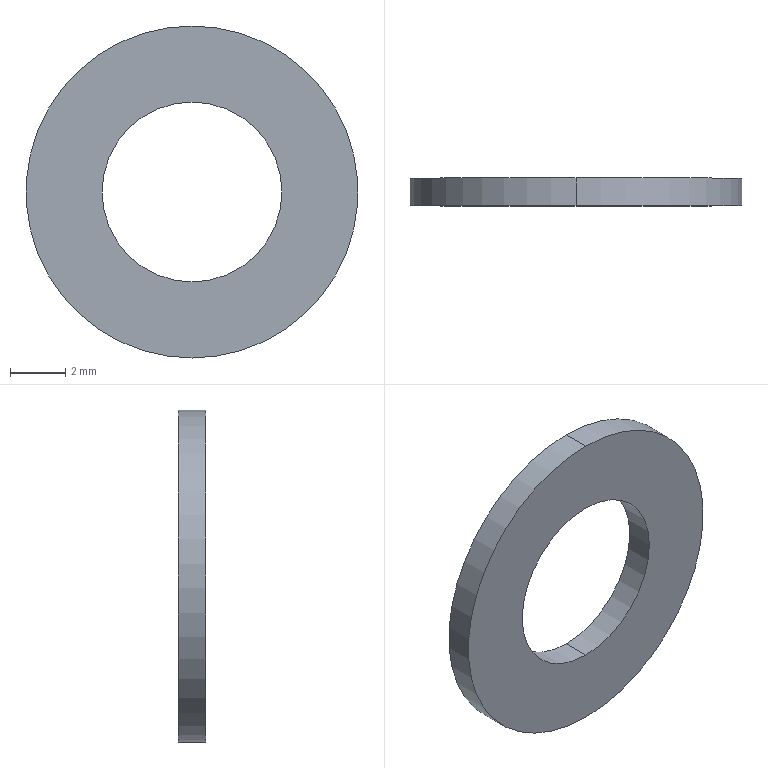Part | STEP file | Washer A | 1 solid | 6 faces | box 12 x 1 x 12 mm | volume 79.914 mm3 | cylinder 4 | plane 2 | commonest cylinder face diameters 6.5 x2 12 x2
STEP:
#1=CARTESIAN_POINT('',(0.,0.,0.));
#2=DIRECTION('',(0.,0.,1.));
#3=DIRECTION('',(1.,0.,0.));
#4=AXIS2_PLACEMENT_3D('',#1,#2,#3);
#5=CARTESIAN_POINT('',(0.,-1.,3.25));
#6=VERTEX_POINT('',#5);
#7=CARTESIAN_POINT('',(0.,0.,3.25));
#8=VERTEX_POINT('',#7);
#9=CARTESIAN_POINT('',(0.,-1.,3.25));
#10=DIRECTION('',(0.,1.,0.));
#11=VECTOR('',#10,1.);
#12=LINE('',#9,#11);
#13=CARTESIAN_POINT('',(0.,-1.,0.));
#14=DIRECTION('',(0.,1.,0.));
#15=DIRECTION('',(0.,0.,1.));
#16=AXIS2_PLACEMENT_3D('',#13,#14,#15);
#17=CYLINDRICAL_SURFACE('',#16,3.25);
#18=CARTESIAN_POINT('',(6.283,0.));
#19=DIRECTION('',(0.,1.));
#20=VECTOR('',#19,1.);
#21=LINE('',#18,#20);
#22=(GEOMETRIC_REPRESENTATION_CONTEXT(2)PARAMETRIC_REPRESENTATION_CONTEXT()REPRESENTATION_CONTEXT('',''));
#23=DEFINITIONAL_REPRESENTATION('',(#21),#22);
#24=PCURVE('',#17,#23);
#25=CARTESIAN_POINT('',(0.,-1.,0.));
#26=DIRECTION('',(0.,1.,0.));
#27=DIRECTION('',(0.,0.,1.));
#28=AXIS2_PLACEMENT_3D('',#25,#26,#27);
#29=CYLINDRICAL_SURFACE('',#28,3.25);
#30=CARTESIAN_POINT('',(0.,0.));
#31=DIRECTION('',(0.,1.));
#32=VECTOR('',#31,1.);
#33=LINE('',#30,#32);
#34=(GEOMETRIC_REPRESENTATION_CONTEXT(2)PARAMETRIC_REPRESENTATION_CONTEXT()REPRESENTATION_CONTEXT('',''));
#35=DEFINITIONAL_REPRESENTATION('',(#33),#34);
#36=PCURVE('',#29,#35);
#37=SURFACE_CURVE('',#12,(#24,#36),.PCURVE_S1.);
#38=EDGE_CURVE('',#6,#8,#37,.T.);
#39=ORIENTED_EDGE('',*,*,#38,.T.);
#40=CARTESIAN_POINT('',(0.,0.,-3.25));
#41=VERTEX_POINT('',#40);
#42=CARTESIAN_POINT('',(0.,0.,0.));
#43=DIRECTION('',(0.,1.,0.));
#44=DIRECTION('',(0.,0.,1.));
#45=AXIS2_PLACEMENT_3D('',#42,#43,#44);
#46=CIRCLE('',#45,3.25);
#47=CARTESIAN_POINT('',(0.,1.));
#48=DIRECTION('',(1.,0.));
#49=VECTOR('',#48,1.);
#50=LINE('',#47,#49);
#51=(GEOMETRIC_REPRESENTATION_CONTEXT(2)PARAMETRIC_REPRESENTATION_CONTEXT()REPRESENTATION_CONTEXT('',''));
#52=DEFINITIONAL_REPRESENTATION('',(#50),#51);
#53=PCURVE('',#17,#52);
#54=CARTESIAN_POINT('',(0.,0.,0.));
#55=DIRECTION('',(0.,1.,0.));
#56=DIRECTION('',(0.,0.,1.));
#57=AXIS2_PLACEMENT_3D('',#54,#55,#56);
#58=PLANE('',#57);
#59=CARTESIAN_POINT('',(0.,0.));
#60=DIRECTION('',(1.,0.));
#61=AXIS2_PLACEMENT_2D('',#59,#60);
#62=CIRCLE('',#61,3.25);
#63=(GEOMETRIC_REPRESENTATION_CONTEXT(2)PARAMETRIC_REPRESENTATION_CONTEXT()REPRESENTATION_CONTEXT('',''));
#64=DEFINITIONAL_REPRESENTATION('',(#62),#63);
#65=PCURVE('',#58,#64);
#66=SURFACE_CURVE('',#46,(#53,#65),.PCURVE_S1.);
#67=EDGE_CURVE('',#41,#8,#66,.T.);
#68=ORIENTED_EDGE('',*,*,#67,.F.);
#69=CARTESIAN_POINT('',(0.,-1.,-3.25));
#70=VERTEX_POINT('',#69);
#71=CARTESIAN_POINT('',(0.,-1.,-3.25));
#72=DIRECTION('',(0.,1.,0.));
#73=VECTOR('',#72,1.);
#74=LINE('',#71,#73);
#75=CARTESIAN_POINT('',(3.142,0.));
#76=DIRECTION('',(0.,1.));
#77=VECTOR('',#76,1.);
#78=LINE('',#75,#77);
#79=(GEOMETRIC_REPRESENTATION_CONTEXT(2)PARAMETRIC_REPRESENTATION_CONTEXT()REPRESENTATION_CONTEXT('',''));
#80=DEFINITIONAL_REPRESENTATION('',(#78),#79);
#81=PCURVE('',#17,#80);
#82=CARTESIAN_POINT('',(3.142,0.));
#83=DIRECTION('',(0.,1.));
#84=VECTOR('',#83,1.);
#85=LINE('',#82,#84);
#86=(GEOMETRIC_REPRESENTATION_CONTEXT(2)PARAMETRIC_REPRESENTATION_CONTEXT()REPRESENTATION_CONTEXT('',''));
#87=DEFINITIONAL_REPRESENTATION('',(#85),#86);
#88=PCURVE('',#29,#87);
#89=SURFACE_CURVE('',#74,(#81,#88),.PCURVE_S1.);
#90=EDGE_CURVE('',#70,#41,#89,.T.);
#91=ORIENTED_EDGE('',*,*,#90,.F.);
#92=CARTESIAN_POINT('',(0.,-1.,0.));
#93=DIRECTION('',(0.,1.,0.));
#94=DIRECTION('',(0.,0.,1.));
#95=AXIS2_PLACEMENT_3D('',#92,#93,#94);
#96=CIRCLE('',#95,3.25);
#97=CARTESIAN_POINT('',(0.,0.));
#98=DIRECTION('',(1.,0.));
#99=VECTOR('',#98,1.);
#100=LINE('',#97,#99);
#101=(GEOMETRIC_REPRESENTATION_CONTEXT(2)PARAMETRIC_REPRESENTATION_CONTEXT()REPRESENTATION_CONTEXT('',''));
#102=DEFINITIONAL_REPRESENTATION('',(#100),#101);
#103=PCURVE('',#17,#102);
#104=CARTESIAN_POINT('',(0.,-1.,0.));
#105=DIRECTION('',(0.,1.,0.));
#106=DIRECTION('',(0.,0.,1.));
#107=AXIS2_PLACEMENT_3D('',#104,#105,#106);
#108=PLANE('',#107);
#109=CARTESIAN_POINT('',(0.,0.));
#110=DIRECTION('',(1.,0.));
#111=AXIS2_PLACEMENT_2D('',#109,#110);
#112=CIRCLE('',#111,3.25);
#113=(GEOMETRIC_REPRESENTATION_CONTEXT(2)PARAMETRIC_REPRESENTATION_CONTEXT()REPRESENTATION_CONTEXT('',''));
#114=DEFINITIONAL_REPRESENTATION('',(#112),#113);
#115=PCURVE('',#108,#114);
#116=SURFACE_CURVE('',#96,(#103,#115),.PCURVE_S1.);
#117=EDGE_CURVE('',#70,#6,#116,.T.);
#118=ORIENTED_EDGE('',*,*,#117,.T.);
#119=EDGE_LOOP('',(#39,#68,#91,#118));
#120=FACE_BOUND('',#119,.F.);
#121=ADVANCED_FACE('',(#120),#17,.F.);
#122=CARTESIAN_POINT('',(0.,-1.,6.));
#123=VERTEX_POINT('',#122);
#124=CARTESIAN_POINT('',(0.,-1.,-6.));
#125=VERTEX_POINT('',#124);
#126=CARTESIAN_POINT('',(0.,-1.,0.));
#127=DIRECTION('',(0.,1.,0.));
#128=DIRECTION('',(0.,0.,1.));
#129=AXIS2_PLACEMENT_3D('',#126,#127,#128);
#130=CIRCLE('',#129,6.);
#131=CARTESIAN_POINT('',(0.,-1.,0.));
#132=DIRECTION('',(0.,1.,0.));
#133=DIRECTION('',(0.,0.,1.));
#134=AXIS2_PLACEMENT_3D('',#131,#132,#133);
#135=CYLINDRICAL_SURFACE('',#134,6.);
#136=CARTESIAN_POINT('',(0.,0.));
#137=DIRECTION('',(1.,0.));
#138=VECTOR('',#137,1.);
#139=LINE('',#136,#138);
#140=(GEOMETRIC_REPRESENTATION_CONTEXT(2)PARAMETRIC_REPRESENTATION_CONTEXT()REPRESENTATION_CONTEXT('',''));
#141=DEFINITIONAL_REPRESENTATION('',(#139),#140);
#142=PCURVE('',#135,#141);
#143=CARTESIAN_POINT('',(0.,0.));
#144=DIRECTION('',(1.,0.));
#145=AXIS2_PLACEMENT_2D('',#143,#144);
#146=CIRCLE('',#145,6.);
#147=(GEOMETRIC_REPRESENTATION_CONTEXT(2)PARAMETRIC_REPRESENTATION_CONTEXT()REPRESENTATION_CONTEXT('',''));
#148=DEFINITIONAL_REPRESENTATION('',(#146),#147);
#149=PCURVE('',#108,#148);
#150=SURFACE_CURVE('',#130,(#142,#149),.PCURVE_S1.);
#151=EDGE_CURVE('',#123,#125,#150,.T.);
#152=ORIENTED_EDGE('',*,*,#151,.T.);
#153=CARTESIAN_POINT('',(0.,0.,-6.));
#154=VERTEX_POINT('',#153);
#155=CARTESIAN_POINT('',(0.,-1.,-6.));
#156=DIRECTION('',(0.,1.,0.));
#157=VECTOR('',#156,1.);
#158=LINE('',#155,#157);
#159=CARTESIAN_POINT('',(3.142,0.));
#160=DIRECTION('',(0.,1.));
#161=VECTOR('',#160,1.);
#162=LINE('',#159,#161);
#163=(GEOMETRIC_REPRESENTATION_CONTEXT(2)PARAMETRIC_REPRESENTATION_CONTEXT()REPRESENTATION_CONTEXT('',''));
#164=DEFINITIONAL_REPRESENTATION('',(#162),#163);
#165=PCURVE('',#135,#164);
#166=CARTESIAN_POINT('',(0.,-1.,0.));
#167=DIRECTION('',(0.,1.,0.));
#168=DIRECTION('',(0.,0.,1.));
#169=AXIS2_PLACEMENT_3D('',#166,#167,#168);
#170=CYLINDRICAL_SURFACE('',#169,6.);
#171=CARTESIAN_POINT('',(3.142,0.));
#172=DIRECTION('',(0.,1.));
#173=VECTOR('',#172,1.);
#174=LINE('',#171,#173);
#175=(GEOMETRIC_REPRESENTATION_CONTEXT(2)PARAMETRIC_REPRESENTATION_CONTEXT()REPRESENTATION_CONTEXT('',''));
#176=DEFINITIONAL_REPRESENTATION('',(#174),#175);
#177=PCURVE('',#170,#176);
#178=SURFACE_CURVE('',#158,(#165,#177),.PCURVE_S1.);
#179=EDGE_CURVE('',#125,#154,#178,.T.);
#180=ORIENTED_EDGE('',*,*,#179,.T.);
#181=CARTESIAN_POINT('',(0.,0.,6.));
#182=VERTEX_POINT('',#181);
#183=CARTESIAN_POINT('',(0.,0.,0.));
#184=DIRECTION('',(0.,1.,0.));
#185=DIRECTION('',(0.,0.,1.));
#186=AXIS2_PLACEMENT_3D('',#183,#184,#185);
#187=CIRCLE('',#186,6.);
#188=CARTESIAN_POINT('',(0.,1.));
#189=DIRECTION('',(1.,0.));
#190=VECTOR('',#189,1.);
#191=LINE('',#188,#190);
#192=(GEOMETRIC_REPRESENTATION_CONTEXT(2)PARAMETRIC_REPRESENTATION_CONTEXT()REPRESENTATION_CONTEXT('',''));
#193=DEFINITIONAL_REPRESENTATION('',(#191),#192);
#194=PCURVE('',#135,#193);
#195=CARTESIAN_POINT('',(0.,0.));
#196=DIRECTION('',(1.,0.));
#197=AXIS2_PLACEMENT_2D('',#195,#196);
#198=CIRCLE('',#197,6.);
#199=(GEOMETRIC_REPRESENTATION_CONTEXT(2)PARAMETRIC_REPRESENTATION_CONTEXT()REPRESENTATION_CONTEXT('',''));
#200=DEFINITIONAL_REPRESENTATION('',(#198),#199);
#201=PCURVE('',#58,#200);
#202=SURFACE_CURVE('',#187,(#194,#201),.PCURVE_S1.);
#203=EDGE_CURVE('',#182,#154,#202,.T.);
#204=ORIENTED_EDGE('',*,*,#203,.F.);
#205=CARTESIAN_POINT('',(0.,-1.,6.));
#206=DIRECTION('',(0.,1.,0.));
#207=VECTOR('',#206,1.);
#208=LINE('',#205,#207);
#209=CARTESIAN_POINT('',(0.,0.));
#210=DIRECTION('',(0.,1.));
#211=VECTOR('',#210,1.);
#212=LINE('',#209,#211);
#213=(GEOMETRIC_REPRESENTATION_CONTEXT(2)PARAMETRIC_REPRESENTATION_CONTEXT()REPRESENTATION_CONTEXT('',''));
#214=DEFINITIONAL_REPRESENTATION('',(#212),#213);
#215=PCURVE('',#135,#214);
#216=CARTESIAN_POINT('',(6.283,0.));
#217=DIRECTION('',(0.,1.));
#218=VECTOR('',#217,1.);
#219=LINE('',#216,#218);
#220=(GEOMETRIC_REPRESENTATION_CONTEXT(2)PARAMETRIC_REPRESENTATION_CONTEXT()REPRESENTATION_CONTEXT('',''));
#221=DEFINITIONAL_REPRESENTATION('',(#219),#220);
#222=PCURVE('',#170,#221);
#223=SURFACE_CURVE('',#208,(#215,#222),.PCURVE_S1.);
#224=EDGE_CURVE('',#123,#182,#223,.T.);
#225=ORIENTED_EDGE('',*,*,#224,.F.);
#226=EDGE_LOOP('',(#152,#180,#204,#225));
#227=FACE_BOUND('',#226,.T.);
#228=ADVANCED_FACE('',(#227),#135,.T.);
#229=ORIENTED_EDGE('',*,*,#179,.F.);
#230=CARTESIAN_POINT('',(0.,-1.,0.));
#231=DIRECTION('',(0.,1.,0.));
#232=DIRECTION('',(0.,0.,1.));
#233=AXIS2_PLACEMENT_3D('',#230,#231,#232);
#234=CIRCLE('',#233,6.);
#235=CARTESIAN_POINT('',(0.,0.));
#236=DIRECTION('',(1.,0.));
#237=VECTOR('',#236,1.);
#238=LINE('',#235,#237);
#239=(GEOMETRIC_REPRESENTATION_CONTEXT(2)PARAMETRIC_REPRESENTATION_CONTEXT()REPRESENTATION_CONTEXT('',''));
#240=DEFINITIONAL_REPRESENTATION('',(#238),#239);
#241=PCURVE('',#170,#240);
#242=CARTESIAN_POINT('',(0.,0.));
#243=DIRECTION('',(1.,0.));
#244=AXIS2_PLACEMENT_2D('',#242,#243);
#245=CIRCLE('',#244,6.);
#246=(GEOMETRIC_REPRESENTATION_CONTEXT(2)PARAMETRIC_REPRESENTATION_CONTEXT()REPRESENTATION_CONTEXT('',''));
#247=DEFINITIONAL_REPRESENTATION('',(#245),#246);
#248=PCURVE('',#108,#247);
#249=SURFACE_CURVE('',#234,(#241,#248),.PCURVE_S1.);
#250=EDGE_CURVE('',#125,#123,#249,.T.);
#251=ORIENTED_EDGE('',*,*,#250,.T.);
#252=ORIENTED_EDGE('',*,*,#224,.T.);
#253=CARTESIAN_POINT('',(0.,0.,0.));
#254=DIRECTION('',(0.,1.,0.));
#255=DIRECTION('',(0.,0.,1.));
#256=AXIS2_PLACEMENT_3D('',#253,#254,#255);
#257=CIRCLE('',#256,6.);
#258=CARTESIAN_POINT('',(0.,1.));
#259=DIRECTION('',(1.,0.));
#260=VECTOR('',#259,1.);
#261=LINE('',#258,#260);
#262=(GEOMETRIC_REPRESENTATION_CONTEXT(2)PARAMETRIC_REPRESENTATION_CONTEXT()REPRESENTATION_CONTEXT('',''));
#263=DEFINITIONAL_REPRESENTATION('',(#261),#262);
#264=PCURVE('',#170,#263);
#265=CARTESIAN_POINT('',(0.,0.));
#266=DIRECTION('',(1.,0.));
#267=AXIS2_PLACEMENT_2D('',#265,#266);
#268=CIRCLE('',#267,6.);
#269=(GEOMETRIC_REPRESENTATION_CONTEXT(2)PARAMETRIC_REPRESENTATION_CONTEXT()REPRESENTATION_CONTEXT('',''));
#270=DEFINITIONAL_REPRESENTATION('',(#268),#269);
#271=PCURVE('',#58,#270);
#272=SURFACE_CURVE('',#257,(#264,#271),.PCURVE_S1.);
#273=EDGE_CURVE('',#154,#182,#272,.T.);
#274=ORIENTED_EDGE('',*,*,#273,.F.);
#275=EDGE_LOOP('',(#229,#251,#252,#274));
#276=FACE_BOUND('',#275,.T.);
#277=ADVANCED_FACE('',(#276),#170,.T.);
#278=CARTESIAN_POINT('',(0.,-1.,0.));
#279=DIRECTION('',(0.,1.,0.));
#280=DIRECTION('',(0.,0.,1.));
#281=AXIS2_PLACEMENT_3D('',#278,#279,#280);
#282=CIRCLE('',#281,3.25);
#283=CARTESIAN_POINT('',(0.,0.));
#284=DIRECTION('',(1.,0.));
#285=AXIS2_PLACEMENT_2D('',#283,#284);
#286=CIRCLE('',#285,3.25);
#287=(GEOMETRIC_REPRESENTATION_CONTEXT(2)PARAMETRIC_REPRESENTATION_CONTEXT()REPRESENTATION_CONTEXT('',''));
#288=DEFINITIONAL_REPRESENTATION('',(#286),#287);
#289=PCURVE('',#108,#288);
#290=CARTESIAN_POINT('',(0.,0.));
#291=DIRECTION('',(1.,0.));
#292=VECTOR('',#291,1.);
#293=LINE('',#290,#292);
#294=(GEOMETRIC_REPRESENTATION_CONTEXT(2)PARAMETRIC_REPRESENTATION_CONTEXT()REPRESENTATION_CONTEXT('',''));
#295=DEFINITIONAL_REPRESENTATION('',(#293),#294);
#296=PCURVE('',#29,#295);
#297=SURFACE_CURVE('',#282,(#289,#296),.PCURVE_S1.);
#298=EDGE_CURVE('',#6,#70,#297,.T.);
#299=ORIENTED_EDGE('',*,*,#298,.T.);
#300=ORIENTED_EDGE('',*,*,#117,.T.);
#301=EDGE_LOOP('',(#299,#300));
#302=FACE_BOUND('',#301,.T.);
#303=ORIENTED_EDGE('',*,*,#151,.F.);
#304=ORIENTED_EDGE('',*,*,#250,.F.);
#305=EDGE_LOOP('',(#303,#304));
#306=FACE_BOUND('',#305,.T.);
#307=ADVANCED_FACE('',(#302,#306),#108,.F.);
#308=CARTESIAN_POINT('',(0.,0.,0.));
#309=DIRECTION('',(0.,1.,0.));
#310=DIRECTION('',(0.,0.,1.));
#311=AXIS2_PLACEMENT_3D('',#308,#309,#310);
#312=CIRCLE('',#311,3.25);
#313=CARTESIAN_POINT('',(0.,0.));
#314=DIRECTION('',(1.,0.));
#315=AXIS2_PLACEMENT_2D('',#313,#314);
#316=CIRCLE('',#315,3.25);
#317=(GEOMETRIC_REPRESENTATION_CONTEXT(2)PARAMETRIC_REPRESENTATION_CONTEXT()REPRESENTATION_CONTEXT('',''));
#318=DEFINITIONAL_REPRESENTATION('',(#316),#317);
#319=PCURVE('',#58,#318);
#320=CARTESIAN_POINT('',(0.,1.));
#321=DIRECTION('',(1.,0.));
#322=VECTOR('',#321,1.);
#323=LINE('',#320,#322);
#324=(GEOMETRIC_REPRESENTATION_CONTEXT(2)PARAMETRIC_REPRESENTATION_CONTEXT()REPRESENTATION_CONTEXT('',''));
#325=DEFINITIONAL_REPRESENTATION('',(#323),#324);
#326=PCURVE('',#29,#325);
#327=SURFACE_CURVE('',#312,(#319,#326),.PCURVE_S1.);
#328=EDGE_CURVE('',#8,#41,#327,.T.);
#329=ORIENTED_EDGE('',*,*,#328,.F.);
#330=ORIENTED_EDGE('',*,*,#67,.F.);
#331=EDGE_LOOP('',(#329,#330));
#332=FACE_BOUND('',#331,.T.);
#333=ORIENTED_EDGE('',*,*,#203,.T.);
#334=ORIENTED_EDGE('',*,*,#273,.T.);
#335=EDGE_LOOP('',(#333,#334));
#336=FACE_BOUND('',#335,.T.);
#337=ADVANCED_FACE('',(#332,#336),#58,.T.);
#338=ORIENTED_EDGE('',*,*,#328,.F.);
#339=ORIENTED_EDGE('',*,*,#38,.F.);
#340=ORIENTED_EDGE('',*,*,#298,.T.);
#341=ORIENTED_EDGE('',*,*,#90,.T.);
#342=EDGE_LOOP('',(#338,#339,#340,#341));
#343=FACE_BOUND('',#342,.F.);
#344=ADVANCED_FACE('',(#343),#29,.F.);
#345=CLOSED_SHELL('',(#121,#228,#277,#307,#337,#344));
#346=MANIFOLD_SOLID_BREP('',#345);
#347=(LENGTH_UNIT()NAMED_UNIT(*)SI_UNIT(.MILLI.,.METRE.));
#348=UNCERTAINTY_MEASURE_WITH_UNIT(LENGTH_MEASURE(0.0000001),#347,'','');
#349=(NAMED_UNIT(*)PLANE_ANGLE_UNIT()SI_UNIT($,.RADIAN.));
#350=(NAMED_UNIT(*)SI_UNIT($,.STERADIAN.)SOLID_ANGLE_UNIT());
#351=(GEOMETRIC_REPRESENTATION_CONTEXT(3)GLOBAL_UNCERTAINTY_ASSIGNED_CONTEXT((#348))GLOBAL_UNIT_ASSIGNED_CONTEXT((#347,#349,#350))REPRESENTATION_CONTEXT('',''));
#352=ADVANCED_BREP_SHAPE_REPRESENTATION('',(#4,#346),#351);